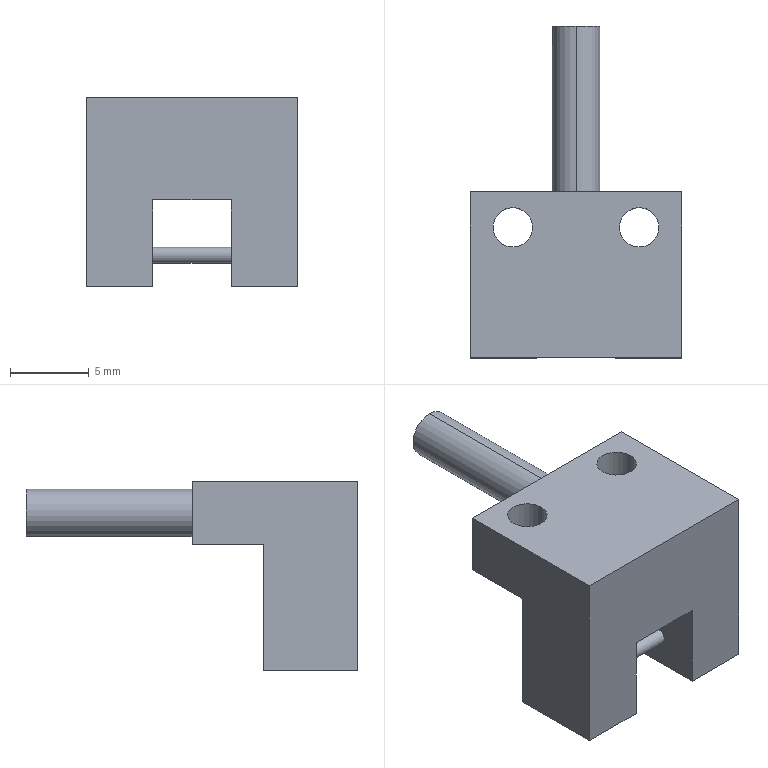Part | SolidWorks | features ICE 4, Extrusion 1 | 1 solid | 21 faces | box 13.4 x 21 x 12 mm | volume 1080 mm3 | plane 13 | cylinder 8 | commonest cylinder face diameters 2.5 x4 1 x2 3 x2
STEP:
#1=CARTESIAN_POINT('',(-2.5,3.,-4.5));
#2=VERTEX_POINT('',#1);
#3=CARTESIAN_POINT('',(-2.5,3.,-3.5));
#4=VERTEX_POINT('',#3);
#5=CARTESIAN_POINT('',(-2.5,3.,-4.));
#6=DIRECTION('',(1.,0.,0.));
#7=DIRECTION('',(0.,0.,1.));
#8=AXIS2_PLACEMENT_3D('',#5,#6,#7);
#9=CIRCLE('',#8,0.5);
#10=EDGE_CURVE('',#2,#4,#9,.T.);
#11=ORIENTED_EDGE('',*,*,#10,.T.);
#12=CARTESIAN_POINT('',(2.5,3.,-3.5));
#13=VERTEX_POINT('',#12);
#14=CARTESIAN_POINT('',(-3.914,3.,-3.5));
#15=DIRECTION('',(1.,0.,0.));
#16=VECTOR('',#15,1000.);
#17=LINE('',#14,#16);
#18=EDGE_CURVE('',#4,#13,#17,.T.);
#19=ORIENTED_EDGE('',*,*,#18,.T.);
#20=CARTESIAN_POINT('',(2.5,3.,-4.5));
#21=VERTEX_POINT('',#20);
#22=CARTESIAN_POINT('',(2.5,3.,-4.));
#23=DIRECTION('',(-1.,0.,0.));
#24=DIRECTION('',(0.,0.,-1.));
#25=AXIS2_PLACEMENT_3D('',#22,#23,#24);
#26=CIRCLE('',#25,0.5);
#27=EDGE_CURVE('',#13,#21,#26,.T.);
#28=ORIENTED_EDGE('',*,*,#27,.T.);
#29=CARTESIAN_POINT('',(-3.914,3.,-4.5));
#30=DIRECTION('',(1.,0.,0.));
#31=VECTOR('',#30,1000.);
#32=LINE('',#29,#31);
#33=EDGE_CURVE('',#2,#21,#32,.T.);
#34=ORIENTED_EDGE('',*,*,#33,.F.);
#35=EDGE_LOOP('',(#11,#19,#28,#34));
#36=FACE_OUTER_BOUND('',#35,.T.);
#37=CARTESIAN_POINT('',(-3.914,3.,-4.));
#38=DIRECTION('',(1.,0.,0.));
#39=DIRECTION('',(0.,0.,-1.));
#40=AXIS2_PLACEMENT_3D('',#37,#38,#39);
#41=CYLINDRICAL_SURFACE('',#40,0.5);
#42=ADVANCED_FACE('',(#36),#41,.T.);
#43=CARTESIAN_POINT('',(-2.75,8.25,6.));
#44=VERTEX_POINT('',#43);
#45=CARTESIAN_POINT('',(-5.25,8.25,6.));
#46=VERTEX_POINT('',#45);
#47=CARTESIAN_POINT('',(-4.,8.25,6.));
#48=DIRECTION('',(0.,0.,-1.));
#49=DIRECTION('',(-1.,0.,0.));
#50=AXIS2_PLACEMENT_3D('',#47,#48,#49);
#51=CIRCLE('',#50,1.25);
#52=EDGE_CURVE('',#44,#46,#51,.T.);
#53=ORIENTED_EDGE('',*,*,#52,.F.);
#54=CARTESIAN_POINT('',(-2.75,8.25,2.));
#55=VERTEX_POINT('',#54);
#56=CARTESIAN_POINT('',(-2.75,8.25,12.5));
#57=DIRECTION('',(0.,0.,-1.));
#58=VECTOR('',#57,1000.);
#59=LINE('',#56,#58);
#60=EDGE_CURVE('',#44,#55,#59,.T.);
#61=ORIENTED_EDGE('',*,*,#60,.T.);
#62=CARTESIAN_POINT('',(-5.25,8.25,2.));
#63=VERTEX_POINT('',#62);
#64=CARTESIAN_POINT('',(-4.,8.25,2.));
#65=DIRECTION('',(0.,0.,-1.));
#66=DIRECTION('',(1.,0.,0.));
#67=AXIS2_PLACEMENT_3D('',#64,#65,#66);
#68=CIRCLE('',#67,1.25);
#69=EDGE_CURVE('',#55,#63,#68,.T.);
#70=ORIENTED_EDGE('',*,*,#69,.T.);
#71=CARTESIAN_POINT('',(-5.25,8.25,12.5));
#72=DIRECTION('',(0.,0.,-1.));
#73=VECTOR('',#72,1000.);
#74=LINE('',#71,#73);
#75=EDGE_CURVE('',#46,#63,#74,.T.);
#76=ORIENTED_EDGE('',*,*,#75,.F.);
#77=EDGE_LOOP('',(#53,#61,#70,#76));
#78=FACE_OUTER_BOUND('',#77,.T.);
#79=CARTESIAN_POINT('',(-4.,8.25,12.5));
#80=DIRECTION('',(0.,0.,-1.));
#81=DIRECTION('',(-1.,0.,0.));
#82=AXIS2_PLACEMENT_3D('',#79,#80,#81);
#83=CYLINDRICAL_SURFACE('',#82,1.25);
#84=ADVANCED_FACE('',(#78),#83,.F.);
#85=CARTESIAN_POINT('',(5.25,8.25,6.));
#86=VERTEX_POINT('',#85);
#87=CARTESIAN_POINT('',(2.75,8.25,6.));
#88=VERTEX_POINT('',#87);
#89=CARTESIAN_POINT('',(4.,8.25,6.));
#90=DIRECTION('',(0.,0.,-1.));
#91=DIRECTION('',(-1.,0.,0.));
#92=AXIS2_PLACEMENT_3D('',#89,#90,#91);
#93=CIRCLE('',#92,1.25);
#94=EDGE_CURVE('',#86,#88,#93,.T.);
#95=ORIENTED_EDGE('',*,*,#94,.F.);
#96=CARTESIAN_POINT('',(5.25,8.25,2.));
#97=VERTEX_POINT('',#96);
#98=CARTESIAN_POINT('',(5.25,8.25,12.5));
#99=DIRECTION('',(0.,0.,-1.));
#100=VECTOR('',#99,1000.);
#101=LINE('',#98,#100);
#102=EDGE_CURVE('',#86,#97,#101,.T.);
#103=ORIENTED_EDGE('',*,*,#102,.T.);
#104=CARTESIAN_POINT('',(2.75,8.25,2.));
#105=VERTEX_POINT('',#104);
#106=CARTESIAN_POINT('',(4.,8.25,2.));
#107=DIRECTION('',(0.,0.,-1.));
#108=DIRECTION('',(-1.,0.,0.));
#109=AXIS2_PLACEMENT_3D('',#106,#107,#108);
#110=CIRCLE('',#109,1.25);
#111=EDGE_CURVE('',#97,#105,#110,.T.);
#112=ORIENTED_EDGE('',*,*,#111,.T.);
#113=CARTESIAN_POINT('',(2.75,8.25,12.5));
#114=DIRECTION('',(0.,0.,-1.));
#115=VECTOR('',#114,1000.);
#116=LINE('',#113,#115);
#117=EDGE_CURVE('',#88,#105,#116,.T.);
#118=ORIENTED_EDGE('',*,*,#117,.F.);
#119=EDGE_LOOP('',(#95,#103,#112,#118));
#120=FACE_OUTER_BOUND('',#119,.T.);
#121=CARTESIAN_POINT('',(4.,8.25,12.5));
#122=DIRECTION('',(0.,0.,-1.));
#123=DIRECTION('',(-1.,0.,0.));
#124=AXIS2_PLACEMENT_3D('',#121,#122,#123);
#125=CYLINDRICAL_SURFACE('',#124,1.25);
#126=ADVANCED_FACE('',(#120),#125,.F.);
#127=CARTESIAN_POINT('',(0.,21.,5.5));
#128=VERTEX_POINT('',#127);
#129=CARTESIAN_POINT('',(0.,21.,2.5));
#130=VERTEX_POINT('',#129);
#131=CARTESIAN_POINT('',(0.,21.,4.));
#132=DIRECTION('',(0.,1.,0.));
#133=DIRECTION('',(0.,0.,1.));
#134=AXIS2_PLACEMENT_3D('',#131,#132,#133);
#135=CIRCLE('',#134,1.5);
#136=EDGE_CURVE('',#128,#130,#135,.T.);
#137=ORIENTED_EDGE('',*,*,#136,.F.);
#138=CARTESIAN_POINT('',(0.,10.5,5.5));
#139=VERTEX_POINT('',#138);
#140=CARTESIAN_POINT('',(0.,21.,5.5));
#141=DIRECTION('',(0.,-1.,0.));
#142=VECTOR('',#141,1000.);
#143=LINE('',#140,#142);
#144=EDGE_CURVE('',#128,#139,#143,.T.);
#145=ORIENTED_EDGE('',*,*,#144,.T.);
#146=CARTESIAN_POINT('',(0.,10.5,2.5));
#147=VERTEX_POINT('',#146);
#148=CARTESIAN_POINT('',(0.,10.5,4.));
#149=DIRECTION('',(0.,1.,0.));
#150=DIRECTION('',(0.,0.,-1.));
#151=AXIS2_PLACEMENT_3D('',#148,#149,#150);
#152=CIRCLE('',#151,1.5);
#153=EDGE_CURVE('',#139,#147,#152,.T.);
#154=ORIENTED_EDGE('',*,*,#153,.T.);
#155=CARTESIAN_POINT('',(0.,21.,2.5));
#156=DIRECTION('',(0.,-1.,0.));
#157=VECTOR('',#156,1000.);
#158=LINE('',#155,#157);
#159=EDGE_CURVE('',#130,#147,#158,.T.);
#160=ORIENTED_EDGE('',*,*,#159,.F.);
#161=EDGE_LOOP('',(#137,#145,#154,#160));
#162=FACE_OUTER_BOUND('',#161,.T.);
#163=CARTESIAN_POINT('',(0.,21.,4.));
#164=DIRECTION('',(0.,-1.,0.));
#165=DIRECTION('',(0.,0.,-1.));
#166=AXIS2_PLACEMENT_3D('',#163,#164,#165);
#167=CYLINDRICAL_SURFACE('',#166,1.5);
#168=ADVANCED_FACE('',(#162),#167,.T.);
#169=CARTESIAN_POINT('',(2.5,0.,-6.));
#170=VERTEX_POINT('',#169);
#171=CARTESIAN_POINT('',(2.5,0.,-0.5));
#172=VERTEX_POINT('',#171);
#173=CARTESIAN_POINT('',(2.5,0.,-6.));
#174=DIRECTION('',(0.,0.,1.));
#175=VECTOR('',#174,1000.);
#176=LINE('',#173,#175);
#177=EDGE_CURVE('',#170,#172,#176,.T.);
#178=ORIENTED_EDGE('',*,*,#177,.T.);
#179=CARTESIAN_POINT('',(2.5,6.,-0.5));
#180=VERTEX_POINT('',#179);
#181=CARTESIAN_POINT('',(2.5,6.,-0.5));
#182=DIRECTION('',(0.,-1.,0.));
#183=VECTOR('',#182,1000.);
#184=LINE('',#181,#183);
#185=EDGE_CURVE('',#180,#172,#184,.T.);
#186=ORIENTED_EDGE('',*,*,#185,.F.);
#187=CARTESIAN_POINT('',(2.5,6.,-6.));
#188=VERTEX_POINT('',#187);
#189=CARTESIAN_POINT('',(2.5,6.,-6.));
#190=DIRECTION('',(0.,0.,1.));
#191=VECTOR('',#190,1000.);
#192=LINE('',#189,#191);
#193=EDGE_CURVE('',#188,#180,#192,.T.);
#194=ORIENTED_EDGE('',*,*,#193,.F.);
#195=CARTESIAN_POINT('',(2.5,6.,-6.));
#196=DIRECTION('',(0.,-1.,0.));
#197=VECTOR('',#196,1000.);
#198=LINE('',#195,#197);
#199=EDGE_CURVE('',#188,#170,#198,.T.);
#200=ORIENTED_EDGE('',*,*,#199,.T.);
#201=EDGE_LOOP('',(#178,#186,#194,#200));
#202=FACE_OUTER_BOUND('',#201,.T.);
#203=CARTESIAN_POINT('',(2.5,3.,-4.));
#204=DIRECTION('',(-1.,0.,0.));
#205=DIRECTION('',(0.,0.,-1.));
#206=AXIS2_PLACEMENT_3D('',#203,#204,#205);
#207=CIRCLE('',#206,0.5);
#208=EDGE_CURVE('',#21,#13,#207,.T.);
#209=ORIENTED_EDGE('',*,*,#208,.F.);
#210=ORIENTED_EDGE('',*,*,#27,.F.);
#211=EDGE_LOOP('',(#209,#210));
#212=FACE_BOUND('',#211,.T.);
#213=CARTESIAN_POINT('',(2.5,6.,-6.));
#214=DIRECTION('',(1.,0.,0.));
#215=DIRECTION('',(0.,0.,-1.));
#216=AXIS2_PLACEMENT_3D('',#213,#214,#215);
#217=PLANE('',#216);
#218=ADVANCED_FACE('',(#202,#212),#217,.F.);
#219=CARTESIAN_POINT('',(-2.5,0.,-0.5));
#220=VERTEX_POINT('',#219);
#221=CARTESIAN_POINT('',(-2.5,0.,-6.));
#222=VERTEX_POINT('',#221);
#223=CARTESIAN_POINT('',(-2.5,0.,-6.));
#224=DIRECTION('',(0.,0.,-1.));
#225=VECTOR('',#224,1000.);
#226=LINE('',#223,#225);
#227=EDGE_CURVE('',#220,#222,#226,.T.);
#228=ORIENTED_EDGE('',*,*,#227,.T.);
#229=CARTESIAN_POINT('',(-2.5,6.,-6.));
#230=VERTEX_POINT('',#229);
#231=CARTESIAN_POINT('',(-2.5,6.,-6.));
#232=DIRECTION('',(0.,-1.,0.));
#233=VECTOR('',#232,1000.);
#234=LINE('',#231,#233);
#235=EDGE_CURVE('',#230,#222,#234,.T.);
#236=ORIENTED_EDGE('',*,*,#235,.F.);
#237=CARTESIAN_POINT('',(-2.5,6.,-0.5));
#238=VERTEX_POINT('',#237);
#239=CARTESIAN_POINT('',(-2.5,6.,-6.));
#240=DIRECTION('',(0.,0.,-1.));
#241=VECTOR('',#240,1000.);
#242=LINE('',#239,#241);
#243=EDGE_CURVE('',#238,#230,#242,.T.);
#244=ORIENTED_EDGE('',*,*,#243,.F.);
#245=CARTESIAN_POINT('',(-2.5,6.,-0.5));
#246=DIRECTION('',(0.,-1.,0.));
#247=VECTOR('',#246,1000.);
#248=LINE('',#245,#247);
#249=EDGE_CURVE('',#238,#220,#248,.T.);
#250=ORIENTED_EDGE('',*,*,#249,.T.);
#251=EDGE_LOOP('',(#228,#236,#244,#250));
#252=FACE_OUTER_BOUND('',#251,.T.);
#253=ORIENTED_EDGE('',*,*,#10,.F.);
#254=CARTESIAN_POINT('',(-2.5,3.,-4.));
#255=DIRECTION('',(1.,0.,0.));
#256=DIRECTION('',(0.,0.,1.));
#257=AXIS2_PLACEMENT_3D('',#254,#255,#256);
#258=CIRCLE('',#257,0.5);
#259=EDGE_CURVE('',#4,#2,#258,.T.);
#260=ORIENTED_EDGE('',*,*,#259,.F.);
#261=EDGE_LOOP('',(#253,#260));
#262=FACE_BOUND('',#261,.T.);
#263=CARTESIAN_POINT('',(-2.5,6.,-6.));
#264=DIRECTION('',(-1.,0.,0.));
#265=DIRECTION('',(0.,0.,1.));
#266=AXIS2_PLACEMENT_3D('',#263,#264,#265);
#267=PLANE('',#266);
#268=ADVANCED_FACE('',(#252,#262),#267,.F.);
#269=CARTESIAN_POINT('',(-6.7,10.5,2.));
#270=VERTEX_POINT('',#269);
#271=CARTESIAN_POINT('',(-6.7,10.5,6.));
#272=VERTEX_POINT('',#271);
#273=CARTESIAN_POINT('',(-6.7,10.5,6.));
#274=DIRECTION('',(0.,0.,1.));
#275=VECTOR('',#274,1000.);
#276=LINE('',#273,#275);
#277=EDGE_CURVE('',#270,#272,#276,.T.);
#278=ORIENTED_EDGE('',*,*,#277,.T.);
#279=CARTESIAN_POINT('',(6.7,10.5,6.));
#280=VERTEX_POINT('',#279);
#281=CARTESIAN_POINT('',(-6.7,10.5,6.));
#282=DIRECTION('',(1.,0.,0.));
#283=VECTOR('',#282,1000.);
#284=LINE('',#281,#283);
#285=EDGE_CURVE('',#272,#280,#284,.T.);
#286=ORIENTED_EDGE('',*,*,#285,.T.);
#287=CARTESIAN_POINT('',(6.7,10.5,2.));
#288=VERTEX_POINT('',#287);
#289=CARTESIAN_POINT('',(6.7,10.5,6.));
#290=DIRECTION('',(0.,0.,-1.));
#291=VECTOR('',#290,1000.);
#292=LINE('',#289,#291);
#293=EDGE_CURVE('',#280,#288,#292,.T.);
#294=ORIENTED_EDGE('',*,*,#293,.T.);
#295=CARTESIAN_POINT('',(-6.7,10.5,2.));
#296=DIRECTION('',(-1.,0.,0.));
#297=VECTOR('',#296,1000.);
#298=LINE('',#295,#297);
#299=EDGE_CURVE('',#288,#270,#298,.T.);
#300=ORIENTED_EDGE('',*,*,#299,.T.);
#301=EDGE_LOOP('',(#278,#286,#294,#300));
#302=FACE_OUTER_BOUND('',#301,.T.);
#303=CARTESIAN_POINT('',(0.,10.5,4.));
#304=DIRECTION('',(0.,1.,0.));
#305=DIRECTION('',(0.,0.,-1.));
#306=AXIS2_PLACEMENT_3D('',#303,#304,#305);
#307=CIRCLE('',#306,1.5);
#308=EDGE_CURVE('',#147,#139,#307,.T.);
#309=ORIENTED_EDGE('',*,*,#308,.F.);
#310=ORIENTED_EDGE('',*,*,#153,.F.);
#311=EDGE_LOOP('',(#309,#310));
#312=FACE_BOUND('',#311,.T.);
#313=CARTESIAN_POINT('',(0.,10.5,0.));
#314=DIRECTION('',(0.,-1.,0.));
#315=DIRECTION('',(0.,0.,-1.));
#316=AXIS2_PLACEMENT_3D('',#313,#314,#315);
#317=PLANE('',#316);
#318=ADVANCED_FACE('',(#302,#312),#317,.F.);
#319=CARTESIAN_POINT('',(6.7,0.,6.));
#320=VERTEX_POINT('',#319);
#321=CARTESIAN_POINT('',(6.7,0.,-6.));
#322=VERTEX_POINT('',#321);
#323=CARTESIAN_POINT('',(6.7,0.,-6.));
#324=DIRECTION('',(0.,0.,-1.));
#325=VECTOR('',#324,1000.);
#326=LINE('',#323,#325);
#327=EDGE_CURVE('',#320,#322,#326,.T.);
#328=ORIENTED_EDGE('',*,*,#327,.T.);
#329=CARTESIAN_POINT('',(6.7,6.,-6.));
#330=VERTEX_POINT('',#329);
#331=CARTESIAN_POINT('',(6.7,6.,-6.));
#332=DIRECTION('',(0.,-1.,0.));
#333=VECTOR('',#332,1000.);
#334=LINE('',#331,#333);
#335=EDGE_CURVE('',#330,#322,#334,.T.);
#336=ORIENTED_EDGE('',*,*,#335,.F.);
#337=CARTESIAN_POINT('',(6.7,6.,2.));
#338=VERTEX_POINT('',#337);
#339=CARTESIAN_POINT('',(6.7,6.,-6.));
#340=DIRECTION('',(0.,0.,-1.));
#341=VECTOR('',#340,1000.);
#342=LINE('',#339,#341);
#343=EDGE_CURVE('',#338,#330,#342,.T.);
#344=ORIENTED_EDGE('',*,*,#343,.F.);
#345=CARTESIAN_POINT('',(6.7,10.5,2.));
#346=DIRECTION('',(0.,-1.,0.));
#347=VECTOR('',#346,1000.);
#348=LINE('',#345,#347);
#349=EDGE_CURVE('',#288,#338,#348,.T.);
#350=ORIENTED_EDGE('',*,*,#349,.F.);
#351=ORIENTED_EDGE('',*,*,#293,.F.);
#352=CARTESIAN_POINT('',(6.7,6.,6.));
#353=DIRECTION('',(0.,-1.,0.));
#354=VECTOR('',#353,1000.);
#355=LINE('',#352,#354);
#356=EDGE_CURVE('',#280,#320,#355,.T.);
#357=ORIENTED_EDGE('',*,*,#356,.T.);
#358=EDGE_LOOP('',(#328,#336,#344,#350,#351,#357));
#359=FACE_OUTER_BOUND('',#358,.T.);
#360=CARTESIAN_POINT('',(6.7,6.,-6.));
#361=DIRECTION('',(-1.,0.,0.));
#362=DIRECTION('',(0.,0.,1.));
#363=AXIS2_PLACEMENT_3D('',#360,#361,#362);
#364=PLANE('',#363);
#365=ADVANCED_FACE('',(#359),#364,.F.);
#366=CARTESIAN_POINT('',(2.5,0.,-6.));
#367=DIRECTION('',(-1.,0.,0.));
#368=VECTOR('',#367,1000.);
#369=LINE('',#366,#368);
#370=EDGE_CURVE('',#322,#170,#369,.T.);
#371=ORIENTED_EDGE('',*,*,#370,.T.);
#372=ORIENTED_EDGE('',*,*,#199,.F.);
#373=CARTESIAN_POINT('',(2.5,6.,-6.));
#374=DIRECTION('',(-1.,0.,0.));
#375=VECTOR('',#374,1000.);
#376=LINE('',#373,#375);
#377=EDGE_CURVE('',#330,#188,#376,.T.);
#378=ORIENTED_EDGE('',*,*,#377,.F.);
#379=ORIENTED_EDGE('',*,*,#335,.T.);
#380=EDGE_LOOP('',(#371,#372,#378,#379));
#381=FACE_OUTER_BOUND('',#380,.T.);
#382=CARTESIAN_POINT('',(2.5,6.,-6.));
#383=DIRECTION('',(0.,0.,1.));
#384=DIRECTION('',(1.,0.,0.));
#385=AXIS2_PLACEMENT_3D('',#382,#383,#384);
#386=PLANE('',#385);
#387=ADVANCED_FACE('',(#381),#386,.F.);
#388=CARTESIAN_POINT('',(-2.5,0.,-0.5));
#389=DIRECTION('',(-1.,0.,0.));
#390=VECTOR('',#389,1000.);
#391=LINE('',#388,#390);
#392=EDGE_CURVE('',#172,#220,#391,.T.);
#393=ORIENTED_EDGE('',*,*,#392,.T.);
#394=ORIENTED_EDGE('',*,*,#249,.F.);
#395=CARTESIAN_POINT('',(-2.5,6.,-0.5));
#396=DIRECTION('',(-1.,0.,0.));
#397=VECTOR('',#396,1000.);
#398=LINE('',#395,#397);
#399=EDGE_CURVE('',#180,#238,#398,.T.);
#400=ORIENTED_EDGE('',*,*,#399,.F.);
#401=ORIENTED_EDGE('',*,*,#185,.T.);
#402=EDGE_LOOP('',(#393,#394,#400,#401));
#403=FACE_OUTER_BOUND('',#402,.T.);
#404=CARTESIAN_POINT('',(-2.5,6.,-0.5));
#405=DIRECTION('',(0.,0.,1.));
#406=DIRECTION('',(1.,0.,0.));
#407=AXIS2_PLACEMENT_3D('',#404,#405,#406);
#408=PLANE('',#407);
#409=ADVANCED_FACE('',(#403),#408,.F.);
#410=CARTESIAN_POINT('',(-6.7,0.,-6.));
#411=VERTEX_POINT('',#410);
#412=CARTESIAN_POINT('',(-6.7,0.,-6.));
#413=DIRECTION('',(-1.,0.,0.));
#414=VECTOR('',#413,1000.);
#415=LINE('',#412,#414);
#416=EDGE_CURVE('',#222,#411,#415,.T.);
#417=ORIENTED_EDGE('',*,*,#416,.T.);
#418=CARTESIAN_POINT('',(-6.7,6.,-6.));
#419=VERTEX_POINT('',#418);
#420=CARTESIAN_POINT('',(-6.7,6.,-6.));
#421=DIRECTION('',(0.,-1.,0.));
#422=VECTOR('',#421,1000.);
#423=LINE('',#420,#422);
#424=EDGE_CURVE('',#419,#411,#423,.T.);
#425=ORIENTED_EDGE('',*,*,#424,.F.);
#426=CARTESIAN_POINT('',(-6.7,6.,-6.));
#427=DIRECTION('',(-1.,0.,0.));
#428=VECTOR('',#427,1000.);
#429=LINE('',#426,#428);
#430=EDGE_CURVE('',#230,#419,#429,.T.);
#431=ORIENTED_EDGE('',*,*,#430,.F.);
#432=ORIENTED_EDGE('',*,*,#235,.T.);
#433=EDGE_LOOP('',(#417,#425,#431,#432));
#434=FACE_OUTER_BOUND('',#433,.T.);
#435=CARTESIAN_POINT('',(-6.7,6.,-6.));
#436=DIRECTION('',(0.,0.,1.));
#437=DIRECTION('',(1.,0.,0.));
#438=AXIS2_PLACEMENT_3D('',#435,#436,#437);
#439=PLANE('',#438);
#440=ADVANCED_FACE('',(#434),#439,.F.);
#441=CARTESIAN_POINT('',(-6.7,0.,6.));
#442=VERTEX_POINT('',#441);
#443=CARTESIAN_POINT('',(-6.7,0.,-6.));
#444=DIRECTION('',(0.,0.,1.));
#445=VECTOR('',#444,1000.);
#446=LINE('',#443,#445);
#447=EDGE_CURVE('',#411,#442,#446,.T.);
#448=ORIENTED_EDGE('',*,*,#447,.T.);
#449=CARTESIAN_POINT('',(-6.7,6.,6.));
#450=DIRECTION('',(0.,-1.,0.));
#451=VECTOR('',#450,1000.);
#452=LINE('',#449,#451);
#453=EDGE_CURVE('',#272,#442,#452,.T.);
#454=ORIENTED_EDGE('',*,*,#453,.F.);
#455=ORIENTED_EDGE('',*,*,#277,.F.);
#456=CARTESIAN_POINT('',(-6.7,6.,2.));
#457=VERTEX_POINT('',#456);
#458=CARTESIAN_POINT('',(-6.7,10.5,2.));
#459=DIRECTION('',(0.,-1.,0.));
#460=VECTOR('',#459,1000.);
#461=LINE('',#458,#460);
#462=EDGE_CURVE('',#270,#457,#461,.T.);
#463=ORIENTED_EDGE('',*,*,#462,.T.);
#464=CARTESIAN_POINT('',(-6.7,6.,-6.));
#465=DIRECTION('',(0.,0.,1.));
#466=VECTOR('',#465,1000.);
#467=LINE('',#464,#466);
#468=EDGE_CURVE('',#419,#457,#467,.T.);
#469=ORIENTED_EDGE('',*,*,#468,.F.);
#470=ORIENTED_EDGE('',*,*,#424,.T.);
#471=EDGE_LOOP('',(#448,#454,#455,#463,#469,#470));
#472=FACE_OUTER_BOUND('',#471,.T.);
#473=CARTESIAN_POINT('',(-6.7,6.,-6.));
#474=DIRECTION('',(1.,0.,0.));
#475=DIRECTION('',(0.,0.,-1.));
#476=AXIS2_PLACEMENT_3D('',#473,#474,#475);
#477=PLANE('',#476);
#478=ADVANCED_FACE('',(#472),#477,.F.);
#479=CARTESIAN_POINT('',(-4.,8.25,6.));
#480=DIRECTION('',(0.,0.,-1.));
#481=DIRECTION('',(-1.,0.,0.));
#482=AXIS2_PLACEMENT_3D('',#479,#480,#481);
#483=CIRCLE('',#482,1.25);
#484=EDGE_CURVE('',#46,#44,#483,.T.);
#485=ORIENTED_EDGE('',*,*,#484,.T.);
#486=ORIENTED_EDGE('',*,*,#52,.T.);
#487=EDGE_LOOP('',(#485,#486));
#488=FACE_BOUND('',#487,.T.);
#489=CARTESIAN_POINT('',(4.,8.25,6.));
#490=DIRECTION('',(0.,0.,-1.));
#491=DIRECTION('',(-1.,0.,0.));
#492=AXIS2_PLACEMENT_3D('',#489,#490,#491);
#493=CIRCLE('',#492,1.25);
#494=EDGE_CURVE('',#88,#86,#493,.T.);
#495=ORIENTED_EDGE('',*,*,#494,.T.);
#496=ORIENTED_EDGE('',*,*,#94,.T.);
#497=EDGE_LOOP('',(#495,#496));
#498=FACE_BOUND('',#497,.T.);
#499=CARTESIAN_POINT('',(-6.7,0.,6.));
#500=DIRECTION('',(1.,0.,0.));
#501=VECTOR('',#500,1000.);
#502=LINE('',#499,#501);
#503=EDGE_CURVE('',#442,#320,#502,.T.);
#504=ORIENTED_EDGE('',*,*,#503,.T.);
#505=ORIENTED_EDGE('',*,*,#356,.F.);
#506=ORIENTED_EDGE('',*,*,#285,.F.);
#507=ORIENTED_EDGE('',*,*,#453,.T.);
#508=EDGE_LOOP('',(#504,#505,#506,#507));
#509=FACE_OUTER_BOUND('',#508,.T.);
#510=CARTESIAN_POINT('',(-6.7,6.,6.));
#511=DIRECTION('',(0.,0.,-1.));
#512=DIRECTION('',(-1.,0.,0.));
#513=AXIS2_PLACEMENT_3D('',#510,#511,#512);
#514=PLANE('',#513);
#515=ADVANCED_FACE('',(#488,#498,#509),#514,.F.);
#516=CARTESIAN_POINT('',(-6.7,6.,2.));
#517=DIRECTION('',(-1.,0.,0.));
#518=VECTOR('',#517,1000.);
#519=LINE('',#516,#518);
#520=EDGE_CURVE('',#338,#457,#519,.T.);
#521=ORIENTED_EDGE('',*,*,#520,.F.);
#522=ORIENTED_EDGE('',*,*,#343,.T.);
#523=ORIENTED_EDGE('',*,*,#377,.T.);
#524=ORIENTED_EDGE('',*,*,#193,.T.);
#525=ORIENTED_EDGE('',*,*,#399,.T.);
#526=ORIENTED_EDGE('',*,*,#243,.T.);
#527=ORIENTED_EDGE('',*,*,#430,.T.);
#528=ORIENTED_EDGE('',*,*,#468,.T.);
#529=EDGE_LOOP('',(#521,#522,#523,#524,#525,#526,#527,#528));
#530=FACE_OUTER_BOUND('',#529,.T.);
#531=CARTESIAN_POINT('',(0.,6.,0.));
#532=DIRECTION('',(0.,1.,0.));
#533=DIRECTION('',(0.,0.,1.));
#534=AXIS2_PLACEMENT_3D('',#531,#532,#533);
#535=PLANE('',#534);
#536=ADVANCED_FACE('',(#530),#535,.T.);
#537=ORIENTED_EDGE('',*,*,#327,.F.);
#538=ORIENTED_EDGE('',*,*,#503,.F.);
#539=ORIENTED_EDGE('',*,*,#447,.F.);
#540=ORIENTED_EDGE('',*,*,#416,.F.);
#541=ORIENTED_EDGE('',*,*,#227,.F.);
#542=ORIENTED_EDGE('',*,*,#392,.F.);
#543=ORIENTED_EDGE('',*,*,#177,.F.);
#544=ORIENTED_EDGE('',*,*,#370,.F.);
#545=EDGE_LOOP('',(#537,#538,#539,#540,#541,#542,#543,#544));
#546=FACE_OUTER_BOUND('',#545,.T.);
#547=CARTESIAN_POINT('',(0.,0.,0.));
#548=DIRECTION('',(0.,1.,0.));
#549=DIRECTION('',(0.,0.,1.));
#550=AXIS2_PLACEMENT_3D('',#547,#548,#549);
#551=PLANE('',#550);
#552=ADVANCED_FACE('',(#546),#551,.F.);
#553=CARTESIAN_POINT('',(-4.,8.25,2.));
#554=DIRECTION('',(0.,0.,-1.));
#555=DIRECTION('',(1.,0.,0.));
#556=AXIS2_PLACEMENT_3D('',#553,#554,#555);
#557=CIRCLE('',#556,1.25);
#558=EDGE_CURVE('',#63,#55,#557,.T.);
#559=ORIENTED_EDGE('',*,*,#558,.F.);
#560=ORIENTED_EDGE('',*,*,#69,.F.);
#561=EDGE_LOOP('',(#559,#560));
#562=FACE_BOUND('',#561,.T.);
#563=CARTESIAN_POINT('',(4.,8.25,2.));
#564=DIRECTION('',(0.,0.,-1.));
#565=DIRECTION('',(-1.,0.,0.));
#566=AXIS2_PLACEMENT_3D('',#563,#564,#565);
#567=CIRCLE('',#566,1.25);
#568=EDGE_CURVE('',#105,#97,#567,.T.);
#569=ORIENTED_EDGE('',*,*,#568,.F.);
#570=ORIENTED_EDGE('',*,*,#111,.F.);
#571=EDGE_LOOP('',(#569,#570));
#572=FACE_BOUND('',#571,.T.);
#573=ORIENTED_EDGE('',*,*,#520,.T.);
#574=ORIENTED_EDGE('',*,*,#462,.F.);
#575=ORIENTED_EDGE('',*,*,#299,.F.);
#576=ORIENTED_EDGE('',*,*,#349,.T.);
#577=EDGE_LOOP('',(#573,#574,#575,#576));
#578=FACE_OUTER_BOUND('',#577,.T.);
#579=CARTESIAN_POINT('',(-6.7,10.5,2.));
#580=DIRECTION('',(0.,0.,1.));
#581=DIRECTION('',(1.,0.,0.));
#582=AXIS2_PLACEMENT_3D('',#579,#580,#581);
#583=PLANE('',#582);
#584=ADVANCED_FACE('',(#562,#572,#578),#583,.F.);
#585=ORIENTED_EDGE('',*,*,#144,.F.);
#586=CARTESIAN_POINT('',(0.,21.,4.));
#587=DIRECTION('',(0.,1.,0.));
#588=DIRECTION('',(0.,0.,1.));
#589=AXIS2_PLACEMENT_3D('',#586,#587,#588);
#590=CIRCLE('',#589,1.5);
#591=EDGE_CURVE('',#130,#128,#590,.T.);
#592=ORIENTED_EDGE('',*,*,#591,.F.);
#593=ORIENTED_EDGE('',*,*,#159,.T.);
#594=ORIENTED_EDGE('',*,*,#308,.T.);
#595=EDGE_LOOP('',(#585,#592,#593,#594));
#596=FACE_OUTER_BOUND('',#595,.T.);
#597=CARTESIAN_POINT('',(0.,21.,4.));
#598=DIRECTION('',(0.,-1.,0.));
#599=DIRECTION('',(0.,0.,-1.));
#600=AXIS2_PLACEMENT_3D('',#597,#598,#599);
#601=CYLINDRICAL_SURFACE('',#600,1.5);
#602=ADVANCED_FACE('',(#596),#601,.T.);
#603=ORIENTED_EDGE('',*,*,#591,.T.);
#604=ORIENTED_EDGE('',*,*,#136,.T.);
#605=EDGE_LOOP('',(#603,#604));
#606=FACE_OUTER_BOUND('',#605,.T.);
#607=CARTESIAN_POINT('',(0.,21.,4.));
#608=DIRECTION('',(0.,1.,0.));
#609=DIRECTION('',(0.,0.,1.));
#610=AXIS2_PLACEMENT_3D('',#607,#608,#609);
#611=PLANE('',#610);
#612=ADVANCED_FACE('',(#606),#611,.T.);
#613=ORIENTED_EDGE('',*,*,#102,.F.);
#614=ORIENTED_EDGE('',*,*,#494,.F.);
#615=ORIENTED_EDGE('',*,*,#117,.T.);
#616=ORIENTED_EDGE('',*,*,#568,.T.);
#617=EDGE_LOOP('',(#613,#614,#615,#616));
#618=FACE_OUTER_BOUND('',#617,.T.);
#619=CARTESIAN_POINT('',(4.,8.25,12.5));
#620=DIRECTION('',(0.,0.,-1.));
#621=DIRECTION('',(-1.,0.,0.));
#622=AXIS2_PLACEMENT_3D('',#619,#620,#621);
#623=CYLINDRICAL_SURFACE('',#622,1.25);
#624=ADVANCED_FACE('',(#618),#623,.F.);
#625=ORIENTED_EDGE('',*,*,#60,.F.);
#626=ORIENTED_EDGE('',*,*,#484,.F.);
#627=ORIENTED_EDGE('',*,*,#75,.T.);
#628=ORIENTED_EDGE('',*,*,#558,.T.);
#629=EDGE_LOOP('',(#625,#626,#627,#628));
#630=FACE_OUTER_BOUND('',#629,.T.);
#631=CARTESIAN_POINT('',(-4.,8.25,12.5));
#632=DIRECTION('',(0.,0.,-1.));
#633=DIRECTION('',(-1.,0.,0.));
#634=AXIS2_PLACEMENT_3D('',#631,#632,#633);
#635=CYLINDRICAL_SURFACE('',#634,1.25);
#636=ADVANCED_FACE('',(#630),#635,.F.);
#637=ORIENTED_EDGE('',*,*,#18,.F.);
#638=ORIENTED_EDGE('',*,*,#259,.T.);
#639=ORIENTED_EDGE('',*,*,#33,.T.);
#640=ORIENTED_EDGE('',*,*,#208,.T.);
#641=EDGE_LOOP('',(#637,#638,#639,#640));
#642=FACE_OUTER_BOUND('',#641,.T.);
#643=CARTESIAN_POINT('',(-3.914,3.,-4.));
#644=DIRECTION('',(1.,0.,0.));
#645=DIRECTION('',(0.,0.,-1.));
#646=AXIS2_PLACEMENT_3D('',#643,#644,#645);
#647=CYLINDRICAL_SURFACE('',#646,0.5);
#648=ADVANCED_FACE('',(#642),#647,.T.);
#649=CLOSED_SHELL('',(#42,#84,#126,#168,#218,#268,#318,#365,#387,#409,#440,#478,#515,#536,#552,#584,#602,#612,#624,#636,#648));
#650=MANIFOLD_SOLID_BREP('',#649);
#651=CARTESIAN_POINT('',(0.,0.,0.));
#652=DIRECTION('',(0.,0.,1.));
#653=DIRECTION('',(1.,0.,0.));
#654=AXIS2_PLACEMENT_3D('',#651,#652,#653);
#655=(LENGTH_UNIT()NAMED_UNIT(*)SI_UNIT(.MILLI.,.METRE.));
#656=UNCERTAINTY_MEASURE_WITH_UNIT(LENGTH_MEASURE(0.00001),#655,'','');
#657=(NAMED_UNIT(*)PLANE_ANGLE_UNIT()SI_UNIT($,.RADIAN.));
#658=(NAMED_UNIT(*)SI_UNIT($,.STERADIAN.)SOLID_ANGLE_UNIT());
#659=(GEOMETRIC_REPRESENTATION_CONTEXT(3)GLOBAL_UNCERTAINTY_ASSIGNED_CONTEXT((#656))GLOBAL_UNIT_ASSIGNED_CONTEXT((#655,#657,#658))REPRESENTATION_CONTEXT('',''));
#660=ADVANCED_BREP_SHAPE_REPRESENTATION('',(#650,#654),#659);